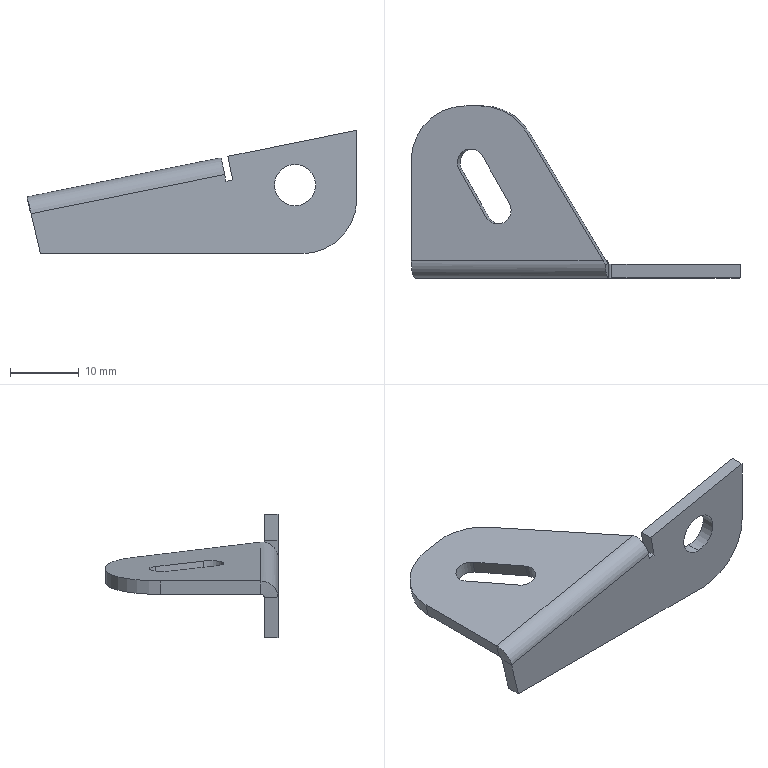Part | SolidWorks | features Fillet 3, ICE 3, Cut 1, EdgeFlange 1, FlatPattern 1, SMBaseFlange 1, SheetMetal 1 | 1 solid | 29 faces | box 48.042 x 25.072 x 17.984 mm | volume 2002 mm3 | plane 18 | cylinder 10 | spline 1 | commonest cylinder face diameters 4 x3 16 x3 6 x2 1 x1 5 x1
STEP:
#1=CARTESIAN_POINT('',(-1.659,15.796,0.3738));
#2=VERTEX_POINT('',#1);
#3=CARTESIAN_POINT('',(-5.317,14.796,-0.3654));
#4=VERTEX_POINT('',#3);
#5=CARTESIAN_POINT('',(-3.357,14.796,0.03071));
#6=DIRECTION('',(-0.1981,0.,0.9802));
#7=DIRECTION('',(-0.9802,0.,-0.1981));
#8=AXIS2_PLACEMENT_3D('',#5,#6,#7);
#9=CIRCLE('',#8,2.);
#10=EDGE_CURVE('',#2,#4,#9,.T.);
#11=ORIENTED_EDGE('',*,*,#10,.T.);
#12=CARTESIAN_POINT('',(-4.921,14.796,-2.326));
#13=VERTEX_POINT('',#12);
#14=CARTESIAN_POINT('',(-6.902,14.796,7.476));
#15=DIRECTION('',(0.1981,0.,-0.9802));
#16=VECTOR('',#15,1000.);
#17=LINE('',#14,#16);
#18=EDGE_CURVE('',#4,#13,#17,.T.);
#19=ORIENTED_EDGE('',*,*,#18,.T.);
#20=CARTESIAN_POINT('',(-1.263,15.796,-1.587));
#21=VERTEX_POINT('',#20);
#22=CARTESIAN_POINT('',(-2.961,14.796,-1.93));
#23=DIRECTION('',(-0.1981,0.,0.9802));
#24=DIRECTION('',(0.9802,0.,0.1981));
#25=AXIS2_PLACEMENT_3D('',#22,#23,#24);
#26=CIRCLE('',#25,2.);
#27=EDGE_CURVE('',#21,#13,#26,.T.);
#28=ORIENTED_EDGE('',*,*,#27,.F.);
#29=CARTESIAN_POINT('',(-3.244,15.796,8.215));
#30=DIRECTION('',(0.1981,0.,-0.9802));
#31=VECTOR('',#30,1000.);
#32=LINE('',#29,#31);
#33=EDGE_CURVE('',#2,#21,#32,.T.);
#34=ORIENTED_EDGE('',*,*,#33,.F.);
#35=EDGE_LOOP('',(#11,#19,#28,#34));
#36=FACE_OUTER_BOUND('',#35,.T.);
#37=CARTESIAN_POINT('',(-4.941,14.796,7.872));
#38=DIRECTION('',(0.1981,0.,-0.9802));
#39=DIRECTION('',(-0.9802,0.,-0.1981));
#40=AXIS2_PLACEMENT_3D('',#37,#38,#39);
#41=CYLINDRICAL_SURFACE('',#40,2.);
#42=ADVANCED_FACE('',(#36),#41,.F.);
#43=CARTESIAN_POINT('',(27.,-2.,-3.));
#44=VERTEX_POINT('',#43);
#45=CARTESIAN_POINT('',(27.,-2.,3.));
#46=VERTEX_POINT('',#45);
#47=CARTESIAN_POINT('',(27.,-2.,0.));
#48=DIRECTION('',(0.,1.,0.));
#49=DIRECTION('',(0.,0.,1.));
#50=AXIS2_PLACEMENT_3D('',#47,#48,#49);
#51=CIRCLE('',#50,3.);
#52=EDGE_CURVE('',#44,#46,#51,.T.);
#53=ORIENTED_EDGE('',*,*,#52,.F.);
#54=CARTESIAN_POINT('',(27.,0.,-3.));
#55=VERTEX_POINT('',#54);
#56=CARTESIAN_POINT('',(27.,-2.,-3.));
#57=DIRECTION('',(0.,1.,0.));
#58=VECTOR('',#57,1000.);
#59=LINE('',#56,#58);
#60=EDGE_CURVE('',#44,#55,#59,.T.);
#61=ORIENTED_EDGE('',*,*,#60,.T.);
#62=CARTESIAN_POINT('',(27.,0.,3.));
#63=VERTEX_POINT('',#62);
#64=CARTESIAN_POINT('',(27.,0.,0.));
#65=DIRECTION('',(0.,1.,0.));
#66=DIRECTION('',(0.,0.,1.));
#67=AXIS2_PLACEMENT_3D('',#64,#65,#66);
#68=CIRCLE('',#67,3.);
#69=EDGE_CURVE('',#55,#63,#68,.T.);
#70=ORIENTED_EDGE('',*,*,#69,.T.);
#71=CARTESIAN_POINT('',(27.,-2.,3.));
#72=DIRECTION('',(0.,1.,0.));
#73=VECTOR('',#72,1000.);
#74=LINE('',#71,#73);
#75=EDGE_CURVE('',#46,#63,#74,.T.);
#76=ORIENTED_EDGE('',*,*,#75,.F.);
#77=EDGE_LOOP('',(#53,#61,#70,#76));
#78=FACE_OUTER_BOUND('',#77,.T.);
#79=CARTESIAN_POINT('',(27.,-2.,0.));
#80=DIRECTION('',(0.,1.,0.));
#81=DIRECTION('',(0.,0.,1.));
#82=AXIS2_PLACEMENT_3D('',#79,#80,#81);
#83=CYLINDRICAL_SURFACE('',#82,3.);
#84=ADVANCED_FACE('',(#78),#83,.F.);
#85=CARTESIAN_POINT('',(15.931,0.5,3.928));
#86=VERTEX_POINT('',#85);
#87=CARTESIAN_POINT('',(4.775,19.227,1.674));
#88=VERTEX_POINT('',#87);
#89=CARTESIAN_POINT('',(11.814,7.411,3.096));
#90=DIRECTION('',(-0.5091,0.8545,-0.1029));
#91=VECTOR('',#90,1000.);
#92=LINE('',#89,#91);
#93=EDGE_CURVE('',#86,#88,#92,.T.);
#94=ORIENTED_EDGE('',*,*,#93,.T.);
#95=CARTESIAN_POINT('',(-1.926,23.072,0.3199));
#96=VERTEX_POINT('',#95);
#97=CARTESIAN_POINT('',(-1.926,15.072,0.3199));
#98=DIRECTION('',(-0.1981,0.,0.9802));
#99=DIRECTION('',(-0.9802,0.,-0.1981));
#100=AXIS2_PLACEMENT_3D('',#97,#98,#99);
#101=CIRCLE('',#100,8.);
#102=EDGE_CURVE('',#88,#96,#101,.T.);
#103=ORIENTED_EDGE('',*,*,#102,.T.);
#104=CARTESIAN_POINT('',(-4.201,23.072,-0.1398));
#105=VERTEX_POINT('',#104);
#106=CARTESIAN_POINT('',(-12.042,23.072,-1.724));
#107=DIRECTION('',(0.9802,0.,0.1981));
#108=VECTOR('',#107,1000.);
#109=LINE('',#106,#108);
#110=EDGE_CURVE('',#105,#96,#109,.T.);
#111=ORIENTED_EDGE('',*,*,#110,.F.);
#112=CARTESIAN_POINT('',(-12.042,15.072,-1.724));
#113=VERTEX_POINT('',#112);
#114=CARTESIAN_POINT('',(-4.201,15.072,-0.1398));
#115=DIRECTION('',(-0.1981,0.,0.9802));
#116=DIRECTION('',(-0.9802,0.,-0.1981));
#117=AXIS2_PLACEMENT_3D('',#114,#115,#116);
#118=CIRCLE('',#117,8.);
#119=EDGE_CURVE('',#105,#113,#118,.T.);
#120=ORIENTED_EDGE('',*,*,#119,.T.);
#121=CARTESIAN_POINT('',(-12.042,0.5,-1.724));
#122=VERTEX_POINT('',#121);
#123=CARTESIAN_POINT('',(-12.042,0.,-1.724));
#124=DIRECTION('',(0.,1.,0.));
#125=VECTOR('',#124,1000.);
#126=LINE('',#123,#125);
#127=EDGE_CURVE('',#122,#113,#126,.T.);
#128=ORIENTED_EDGE('',*,*,#127,.F.);
#129=CARTESIAN_POINT('',(-12.042,0.5,-1.724));
#130=DIRECTION('',(-0.9802,0.,-0.1981));
#131=VECTOR('',#130,1000.);
#132=LINE('',#129,#131);
#133=EDGE_CURVE('',#86,#122,#132,.T.);
#134=ORIENTED_EDGE('',*,*,#133,.F.);
#135=EDGE_LOOP('',(#94,#103,#111,#120,#128,#134));
#136=FACE_OUTER_BOUND('',#135,.T.);
#137=ORIENTED_EDGE('',*,*,#10,.F.);
#138=CARTESIAN_POINT('',(2.262,8.867,1.166));
#139=VERTEX_POINT('',#138);
#140=CARTESIAN_POINT('',(5.425,3.277,1.805));
#141=DIRECTION('',(-0.4901,0.866,-0.09904));
#142=VECTOR('',#141,1000.);
#143=LINE('',#140,#142);
#144=EDGE_CURVE('',#139,#2,#143,.T.);
#145=ORIENTED_EDGE('',*,*,#144,.F.);
#146=CARTESIAN_POINT('',(-1.134,6.867,0.4799));
#147=VERTEX_POINT('',#146);
#148=CARTESIAN_POINT('',(0.564,7.867,0.823));
#149=DIRECTION('',(-0.1981,0.,0.9802));
#150=DIRECTION('',(-0.9802,0.,-0.1981));
#151=AXIS2_PLACEMENT_3D('',#148,#149,#150);
#152=CIRCLE('',#151,2.);
#153=EDGE_CURVE('',#147,#139,#152,.T.);
#154=ORIENTED_EDGE('',*,*,#153,.F.);
#155=CARTESIAN_POINT('',(-5.055,13.796,-0.3124));
#156=VERTEX_POINT('',#155);
#157=CARTESIAN_POINT('',(2.03,1.277,1.119));
#158=DIRECTION('',(0.4901,-0.866,0.09904));
#159=VECTOR('',#158,1000.);
#160=LINE('',#157,#159);
#161=EDGE_CURVE('',#156,#147,#160,.T.);
#162=ORIENTED_EDGE('',*,*,#161,.F.);
#163=CARTESIAN_POINT('',(-3.357,14.796,0.03071));
#164=DIRECTION('',(-0.1981,0.,0.9802));
#165=DIRECTION('',(-0.9802,0.,-0.1981));
#166=AXIS2_PLACEMENT_3D('',#163,#164,#165);
#167=CIRCLE('',#166,2.);
#168=EDGE_CURVE('',#4,#156,#167,.T.);
#169=ORIENTED_EDGE('',*,*,#168,.F.);
#170=EDGE_LOOP('',(#137,#145,#154,#162,#169));
#171=FACE_BOUND('',#170,.T.);
#172=CARTESIAN_POINT('',(-0.1377,0.,0.6812));
#173=DIRECTION('',(0.1981,0.,-0.9802));
#174=DIRECTION('',(-0.9802,0.,-0.1981));
#175=AXIS2_PLACEMENT_3D('',#172,#173,#174);
#176=PLANE('',#175);
#177=ADVANCED_FACE('',(#136,#171),#176,.F.);
#178=CARTESIAN_POINT('',(-3.805,23.072,-2.1));
#179=VERTEX_POINT('',#178);
#180=CARTESIAN_POINT('',(-1.53,23.072,-1.64));
#181=VERTEX_POINT('',#180);
#182=CARTESIAN_POINT('',(0.2585,23.072,-1.279));
#183=DIRECTION('',(0.9802,0.,0.1981));
#184=VECTOR('',#183,1000.);
#185=LINE('',#182,#184);
#186=EDGE_CURVE('',#179,#181,#185,.T.);
#187=ORIENTED_EDGE('',*,*,#186,.T.);
#188=CARTESIAN_POINT('',(5.171,19.227,-0.2864));
#189=VERTEX_POINT('',#188);
#190=CARTESIAN_POINT('',(-1.53,15.072,-1.64));
#191=DIRECTION('',(0.1981,0.,-0.9802));
#192=DIRECTION('',(-0.9802,0.,-0.1981));
#193=AXIS2_PLACEMENT_3D('',#190,#191,#192);
#194=CIRCLE('',#193,8.);
#195=EDGE_CURVE('',#181,#189,#194,.T.);
#196=ORIENTED_EDGE('',*,*,#195,.T.);
#197=CARTESIAN_POINT('',(16.327,0.5,1.968));
#198=VERTEX_POINT('',#197);
#199=CARTESIAN_POINT('',(16.625,0.,2.028));
#200=DIRECTION('',(-0.5091,0.8545,-0.1029));
#201=VECTOR('',#200,1000.);
#202=LINE('',#199,#201);
#203=EDGE_CURVE('',#198,#189,#202,.T.);
#204=ORIENTED_EDGE('',*,*,#203,.F.);
#205=CARTESIAN_POINT('',(-11.646,0.5,-3.685));
#206=VERTEX_POINT('',#205);
#207=CARTESIAN_POINT('',(-11.646,0.5,-3.685));
#208=DIRECTION('',(0.9802,0.,0.1981));
#209=VECTOR('',#208,1000.);
#210=LINE('',#207,#209);
#211=EDGE_CURVE('',#206,#198,#210,.T.);
#212=ORIENTED_EDGE('',*,*,#211,.F.);
#213=CARTESIAN_POINT('',(-11.646,15.072,-3.685));
#214=VERTEX_POINT('',#213);
#215=CARTESIAN_POINT('',(-11.646,0.,-3.685));
#216=DIRECTION('',(0.,1.,0.));
#217=VECTOR('',#216,1000.);
#218=LINE('',#215,#217);
#219=EDGE_CURVE('',#206,#214,#218,.T.);
#220=ORIENTED_EDGE('',*,*,#219,.T.);
#221=CARTESIAN_POINT('',(-3.805,15.072,-2.1));
#222=DIRECTION('',(0.1981,0.,-0.9802));
#223=DIRECTION('',(-0.9802,0.,-0.1981));
#224=AXIS2_PLACEMENT_3D('',#221,#222,#223);
#225=CIRCLE('',#224,8.);
#226=EDGE_CURVE('',#214,#179,#225,.T.);
#227=ORIENTED_EDGE('',*,*,#226,.T.);
#228=EDGE_LOOP('',(#187,#196,#204,#212,#220,#227));
#229=FACE_OUTER_BOUND('',#228,.T.);
#230=CARTESIAN_POINT('',(2.658,8.867,-0.7943));
#231=VERTEX_POINT('',#230);
#232=CARTESIAN_POINT('',(-1.263,15.796,-1.587));
#233=DIRECTION('',(-0.4901,0.866,-0.09904));
#234=VECTOR('',#233,1000.);
#235=LINE('',#232,#234);
#236=EDGE_CURVE('',#231,#21,#235,.T.);
#237=ORIENTED_EDGE('',*,*,#236,.T.);
#238=ORIENTED_EDGE('',*,*,#27,.T.);
#239=CARTESIAN_POINT('',(-4.658,13.796,-2.273));
#240=VERTEX_POINT('',#239);
#241=CARTESIAN_POINT('',(-2.961,14.796,-1.93));
#242=DIRECTION('',(-0.1981,0.,0.9802));
#243=DIRECTION('',(0.9802,0.,0.1981));
#244=AXIS2_PLACEMENT_3D('',#241,#242,#243);
#245=CIRCLE('',#244,2.);
#246=EDGE_CURVE('',#13,#240,#245,.T.);
#247=ORIENTED_EDGE('',*,*,#246,.T.);
#248=CARTESIAN_POINT('',(-0.7376,6.867,-1.48));
#249=VERTEX_POINT('',#248);
#250=CARTESIAN_POINT('',(-4.658,13.796,-2.273));
#251=DIRECTION('',(0.4901,-0.866,0.09904));
#252=VECTOR('',#251,1000.);
#253=LINE('',#250,#252);
#254=EDGE_CURVE('',#240,#249,#253,.T.);
#255=ORIENTED_EDGE('',*,*,#254,.T.);
#256=CARTESIAN_POINT('',(0.9601,7.867,-1.137));
#257=DIRECTION('',(-0.1981,0.,0.9802));
#258=DIRECTION('',(0.9802,0.,0.1981));
#259=AXIS2_PLACEMENT_3D('',#256,#257,#258);
#260=CIRCLE('',#259,2.);
#261=EDGE_CURVE('',#249,#231,#260,.T.);
#262=ORIENTED_EDGE('',*,*,#261,.T.);
#263=EDGE_LOOP('',(#237,#238,#247,#255,#262));
#264=FACE_BOUND('',#263,.T.);
#265=CARTESIAN_POINT('',(0.2585,0.,-1.279));
#266=DIRECTION('',(0.1981,0.,-0.9802));
#267=DIRECTION('',(-0.9802,0.,-0.1981));
#268=AXIS2_PLACEMENT_3D('',#265,#266,#267);
#269=PLANE('',#268);
#270=ADVANCED_FACE('',(#229,#264),#269,.T.);
#271=CARTESIAN_POINT('',(27.,-2.,0.));
#272=DIRECTION('',(0.,1.,0.));
#273=DIRECTION('',(0.,0.,1.));
#274=AXIS2_PLACEMENT_3D('',#271,#272,#273);
#275=CIRCLE('',#274,3.);
#276=EDGE_CURVE('',#46,#44,#275,.T.);
#277=ORIENTED_EDGE('',*,*,#276,.T.);
#278=ORIENTED_EDGE('',*,*,#52,.T.);
#279=EDGE_LOOP('',(#277,#278));
#280=FACE_BOUND('',#279,.T.);
#281=CARTESIAN_POINT('',(28.,-2.,-10.));
#282=VERTEX_POINT('',#281);
#283=CARTESIAN_POINT('',(-10.106,-2.,-10.));
#284=VERTEX_POINT('',#283);
#285=CARTESIAN_POINT('',(-36.,-2.,-10.));
#286=DIRECTION('',(-1.,0.,0.));
#287=VECTOR('',#286,1000.);
#288=LINE('',#285,#287);
#289=EDGE_CURVE('',#282,#284,#288,.T.);
#290=ORIENTED_EDGE('',*,*,#289,.F.);
#291=CARTESIAN_POINT('',(36.,-2.,-2.));
#292=VERTEX_POINT('',#291);
#293=CARTESIAN_POINT('',(28.,-2.,-2.));
#294=DIRECTION('',(0.,-1.,0.));
#295=DIRECTION('',(0.,0.,1.));
#296=AXIS2_PLACEMENT_3D('',#293,#294,#295);
#297=CIRCLE('',#296,8.);
#298=EDGE_CURVE('',#282,#292,#297,.T.);
#299=ORIENTED_EDGE('',*,*,#298,.T.);
#300=CARTESIAN_POINT('',(36.,-2.,7.984));
#301=VERTEX_POINT('',#300);
#302=CARTESIAN_POINT('',(36.,-2.,-10.));
#303=DIRECTION('',(0.,0.,-1.));
#304=VECTOR('',#303,1000.);
#305=LINE('',#302,#304);
#306=EDGE_CURVE('',#301,#292,#305,.T.);
#307=ORIENTED_EDGE('',*,*,#306,.F.);
#308=CARTESIAN_POINT('',(17.209,-2.,4.187));
#309=VERTEX_POINT('',#308);
#310=CARTESIAN_POINT('',(-0.1377,-2.,0.6812));
#311=DIRECTION('',(0.9802,0.,0.1981));
#312=VECTOR('',#311,1000.);
#313=LINE('',#310,#312);
#314=EDGE_CURVE('',#309,#301,#313,.T.);
#315=ORIENTED_EDGE('',*,*,#314,.F.);
#316=CARTESIAN_POINT('',(17.903,-2.,0.756));
#317=VERTEX_POINT('',#316);
#318=CARTESIAN_POINT('',(17.347,-2.,3.505));
#319=DIRECTION('',(-0.1981,0.,0.9802));
#320=VECTOR('',#319,1000.);
#321=LINE('',#318,#320);
#322=EDGE_CURVE('',#317,#309,#321,.T.);
#323=ORIENTED_EDGE('',*,*,#322,.F.);
#324=CARTESIAN_POINT('',(16.922,-2.,0.558));
#325=VERTEX_POINT('',#324);
#326=CARTESIAN_POINT('',(0.5556,-2.,-2.749));
#327=DIRECTION('',(0.9802,0.,0.1981));
#328=VECTOR('',#327,1000.);
#329=LINE('',#326,#328);
#330=EDGE_CURVE('',#325,#317,#329,.T.);
#331=ORIENTED_EDGE('',*,*,#330,.F.);
#332=CARTESIAN_POINT('',(16.724,-2.,1.538));
#333=VERTEX_POINT('',#332);
#334=CARTESIAN_POINT('',(16.367,-2.,3.307));
#335=DIRECTION('',(0.1981,0.,-0.9802));
#336=VECTOR('',#335,1000.);
#337=LINE('',#334,#336);
#338=EDGE_CURVE('',#333,#325,#337,.T.);
#339=ORIENTED_EDGE('',*,*,#338,.F.);
#340=CARTESIAN_POINT('',(-11.473,-2.,-4.16));
#341=VERTEX_POINT('',#340);
#342=CARTESIAN_POINT('',(16.724,-2.,1.538));
#343=DIRECTION('',(-0.9802,0.,-0.1981));
#344=VECTOR('',#343,1000.);
#345=LINE('',#342,#344);
#346=EDGE_CURVE('',#333,#341,#345,.T.);
#347=ORIENTED_EDGE('',*,*,#346,.T.);
#348=CARTESIAN_POINT('',(-11.8,-2.,-2.76));
#349=DIRECTION('',(0.2278,0.,-0.9737));
#350=VECTOR('',#349,1000.);
#351=LINE('',#348,#350);
#352=EDGE_CURVE('',#341,#284,#351,.T.);
#353=ORIENTED_EDGE('',*,*,#352,.T.);
#354=EDGE_LOOP('',(#290,#299,#307,#315,#323,#331,#339,#347,#353));
#355=FACE_OUTER_BOUND('',#354,.T.);
#356=CARTESIAN_POINT('',(0.,-2.,0.));
#357=DIRECTION('',(0.,1.,0.));
#358=DIRECTION('',(0.,0.,1.));
#359=AXIS2_PLACEMENT_3D('',#356,#357,#358);
#360=PLANE('',#359);
#361=ADVANCED_FACE('',(#280,#355),#360,.F.);
#362=CARTESIAN_POINT('',(27.,0.,0.));
#363=DIRECTION('',(0.,1.,0.));
#364=DIRECTION('',(0.,0.,1.));
#365=AXIS2_PLACEMENT_3D('',#362,#363,#364);
#366=CIRCLE('',#365,3.);
#367=EDGE_CURVE('',#63,#55,#366,.T.);
#368=ORIENTED_EDGE('',*,*,#367,.F.);
#369=ORIENTED_EDGE('',*,*,#69,.F.);
#370=EDGE_LOOP('',(#368,#369));
#371=FACE_BOUND('',#370,.T.);
#372=CARTESIAN_POINT('',(36.,0.,7.984));
#373=VERTEX_POINT('',#372);
#374=CARTESIAN_POINT('',(36.,0.,-2.));
#375=VERTEX_POINT('',#374);
#376=CARTESIAN_POINT('',(36.,0.,-10.));
#377=DIRECTION('',(0.,0.,-1.));
#378=VECTOR('',#377,1000.);
#379=LINE('',#376,#378);
#380=EDGE_CURVE('',#373,#375,#379,.T.);
#381=ORIENTED_EDGE('',*,*,#380,.T.);
#382=CARTESIAN_POINT('',(28.,0.,-10.));
#383=VERTEX_POINT('',#382);
#384=CARTESIAN_POINT('',(28.,0.,-2.));
#385=DIRECTION('',(0.,1.,0.));
#386=DIRECTION('',(0.,0.,1.));
#387=AXIS2_PLACEMENT_3D('',#384,#385,#386);
#388=CIRCLE('',#387,8.);
#389=EDGE_CURVE('',#375,#383,#388,.T.);
#390=ORIENTED_EDGE('',*,*,#389,.T.);
#391=CARTESIAN_POINT('',(-10.106,0.,-10.));
#392=VERTEX_POINT('',#391);
#393=CARTESIAN_POINT('',(-36.,0.,-10.));
#394=DIRECTION('',(-1.,0.,0.));
#395=VECTOR('',#394,1000.);
#396=LINE('',#393,#395);
#397=EDGE_CURVE('',#383,#392,#396,.T.);
#398=ORIENTED_EDGE('',*,*,#397,.T.);
#399=CARTESIAN_POINT('',(-11.473,0.,-4.16));
#400=VERTEX_POINT('',#399);
#401=CARTESIAN_POINT('',(-11.8,0.,-2.76));
#402=DIRECTION('',(0.2278,0.,-0.9737));
#403=VECTOR('',#402,1000.);
#404=LINE('',#401,#403);
#405=EDGE_CURVE('',#400,#392,#404,.T.);
#406=ORIENTED_EDGE('',*,*,#405,.F.);
#407=CARTESIAN_POINT('',(16.724,0.,1.538));
#408=VERTEX_POINT('',#407);
#409=CARTESIAN_POINT('',(16.724,0.,1.538));
#410=DIRECTION('',(-0.9802,0.,-0.1981));
#411=VECTOR('',#410,1000.);
#412=LINE('',#409,#411);
#413=EDGE_CURVE('',#408,#400,#412,.T.);
#414=ORIENTED_EDGE('',*,*,#413,.F.);
#415=CARTESIAN_POINT('',(16.922,0.,0.558));
#416=VERTEX_POINT('',#415);
#417=CARTESIAN_POINT('',(16.922,0.,0.558));
#418=DIRECTION('',(-0.1981,0.,0.9802));
#419=VECTOR('',#418,1000.);
#420=LINE('',#417,#419);
#421=EDGE_CURVE('',#416,#408,#420,.T.);
#422=ORIENTED_EDGE('',*,*,#421,.F.);
#423=CARTESIAN_POINT('',(17.903,0.,0.756));
#424=VERTEX_POINT('',#423);
#425=CARTESIAN_POINT('',(17.903,0.,0.756));
#426=DIRECTION('',(-0.9802,0.,-0.1981));
#427=VECTOR('',#426,1000.);
#428=LINE('',#425,#427);
#429=EDGE_CURVE('',#424,#416,#428,.T.);
#430=ORIENTED_EDGE('',*,*,#429,.F.);
#431=CARTESIAN_POINT('',(17.209,0.,4.187));
#432=VERTEX_POINT('',#431);
#433=CARTESIAN_POINT('',(17.209,0.,4.187));
#434=DIRECTION('',(0.1981,0.,-0.9802));
#435=VECTOR('',#434,1000.);
#436=LINE('',#433,#435);
#437=EDGE_CURVE('',#432,#424,#436,.T.);
#438=ORIENTED_EDGE('',*,*,#437,.F.);
#439=CARTESIAN_POINT('',(-0.1377,0.,0.6812));
#440=DIRECTION('',(0.9802,0.,0.1981));
#441=VECTOR('',#440,1000.);
#442=LINE('',#439,#441);
#443=EDGE_CURVE('',#432,#373,#442,.T.);
#444=ORIENTED_EDGE('',*,*,#443,.T.);
#445=EDGE_LOOP('',(#381,#390,#398,#406,#414,#422,#430,#438,#444));
#446=FACE_OUTER_BOUND('',#445,.T.);
#447=CARTESIAN_POINT('',(0.,0.,0.));
#448=DIRECTION('',(0.,1.,0.));
#449=DIRECTION('',(0.,0.,1.));
#450=AXIS2_PLACEMENT_3D('',#447,#448,#449);
#451=PLANE('',#450);
#452=ADVANCED_FACE('',(#371,#446),#451,.T.);
#453=ORIENTED_EDGE('',*,*,#443,.F.);
#454=CARTESIAN_POINT('',(17.209,0.,4.187));
#455=DIRECTION('',(0.,-1.,0.));
#456=VECTOR('',#455,1000.);
#457=LINE('',#454,#456);
#458=EDGE_CURVE('',#432,#309,#457,.T.);
#459=ORIENTED_EDGE('',*,*,#458,.T.);
#460=ORIENTED_EDGE('',*,*,#314,.T.);
#461=CARTESIAN_POINT('',(36.,-10.,7.984));
#462=DIRECTION('',(0.,1.,0.));
#463=VECTOR('',#462,1000.);
#464=LINE('',#461,#463);
#465=EDGE_CURVE('',#301,#373,#464,.T.);
#466=ORIENTED_EDGE('',*,*,#465,.T.);
#467=EDGE_LOOP('',(#453,#459,#460,#466));
#468=FACE_OUTER_BOUND('',#467,.T.);
#469=CARTESIAN_POINT('',(-0.1377,-10.,0.6812));
#470=DIRECTION('',(-0.1981,0.,0.9802));
#471=DIRECTION('',(0.9802,0.,0.1981));
#472=AXIS2_PLACEMENT_3D('',#469,#470,#471);
#473=PLANE('',#472);
#474=ADVANCED_FACE('',(#468),#473,.T.);
#475=CARTESIAN_POINT('',(-11.473,0.,-4.16));
#476=DIRECTION('',(0.,-1.,0.));
#477=VECTOR('',#476,1000.);
#478=LINE('',#475,#477);
#479=EDGE_CURVE('',#400,#341,#478,.T.);
#480=ORIENTED_EDGE('',*,*,#479,.F.);
#481=ORIENTED_EDGE('',*,*,#405,.T.);
#482=CARTESIAN_POINT('',(-10.106,-10.,-10.));
#483=DIRECTION('',(0.,1.,0.));
#484=VECTOR('',#483,1000.);
#485=LINE('',#482,#484);
#486=EDGE_CURVE('',#284,#392,#485,.T.);
#487=ORIENTED_EDGE('',*,*,#486,.F.);
#488=ORIENTED_EDGE('',*,*,#352,.F.);
#489=EDGE_LOOP('',(#480,#481,#487,#488));
#490=FACE_OUTER_BOUND('',#489,.T.);
#491=CARTESIAN_POINT('',(-11.8,-10.,-2.76));
#492=DIRECTION('',(0.9737,0.,0.2278));
#493=DIRECTION('',(0.2278,0.,-0.9737));
#494=AXIS2_PLACEMENT_3D('',#491,#492,#493);
#495=PLANE('',#494);
#496=ADVANCED_FACE('',(#490),#495,.F.);
#497=ORIENTED_EDGE('',*,*,#306,.T.);
#498=CARTESIAN_POINT('',(36.,-2.,-2.));
#499=DIRECTION('',(0.,1.,0.));
#500=VECTOR('',#499,1000.);
#501=LINE('',#498,#500);
#502=EDGE_CURVE('',#292,#375,#501,.T.);
#503=ORIENTED_EDGE('',*,*,#502,.T.);
#504=ORIENTED_EDGE('',*,*,#380,.F.);
#505=ORIENTED_EDGE('',*,*,#465,.F.);
#506=EDGE_LOOP('',(#497,#503,#504,#505));
#507=FACE_OUTER_BOUND('',#506,.T.);
#508=CARTESIAN_POINT('',(36.,-2.,-10.));
#509=DIRECTION('',(1.,0.,0.));
#510=DIRECTION('',(0.,0.,-1.));
#511=AXIS2_PLACEMENT_3D('',#508,#509,#510);
#512=PLANE('',#511);
#513=ADVANCED_FACE('',(#507),#512,.T.);
#514=ORIENTED_EDGE('',*,*,#397,.F.);
#515=CARTESIAN_POINT('',(28.,-2.,-10.));
#516=DIRECTION('',(0.,-1.,0.));
#517=VECTOR('',#516,1000.);
#518=LINE('',#515,#517);
#519=EDGE_CURVE('',#383,#282,#518,.T.);
#520=ORIENTED_EDGE('',*,*,#519,.T.);
#521=ORIENTED_EDGE('',*,*,#289,.T.);
#522=ORIENTED_EDGE('',*,*,#486,.T.);
#523=EDGE_LOOP('',(#514,#520,#521,#522));
#524=FACE_OUTER_BOUND('',#523,.T.);
#525=CARTESIAN_POINT('',(-36.,-2.,-10.));
#526=DIRECTION('',(0.,0.,-1.));
#527=DIRECTION('',(-1.,0.,0.));
#528=AXIS2_PLACEMENT_3D('',#525,#526,#527);
#529=PLANE('',#528);
#530=ADVANCED_FACE('',(#524),#529,.T.);
#531=ORIENTED_EDGE('',*,*,#60,.F.);
#532=ORIENTED_EDGE('',*,*,#276,.F.);
#533=ORIENTED_EDGE('',*,*,#75,.T.);
#534=ORIENTED_EDGE('',*,*,#367,.T.);
#535=EDGE_LOOP('',(#531,#532,#533,#534));
#536=FACE_OUTER_BOUND('',#535,.T.);
#537=CARTESIAN_POINT('',(27.,-2.,0.));
#538=DIRECTION('',(0.,1.,0.));
#539=DIRECTION('',(0.,0.,1.));
#540=AXIS2_PLACEMENT_3D('',#537,#538,#539);
#541=CYLINDRICAL_SURFACE('',#540,3.);
#542=ADVANCED_FACE('',(#536),#541,.F.);
#543=CARTESIAN_POINT('',(16.922,0.,0.558));
#544=DIRECTION('',(0.,-1.,0.));
#545=VECTOR('',#544,1000.);
#546=LINE('',#543,#545);
#547=EDGE_CURVE('',#416,#325,#546,.T.);
#548=ORIENTED_EDGE('',*,*,#547,.T.);
#549=ORIENTED_EDGE('',*,*,#330,.T.);
#550=CARTESIAN_POINT('',(17.903,0.,0.756));
#551=DIRECTION('',(0.,-1.,0.));
#552=VECTOR('',#551,1000.);
#553=LINE('',#550,#552);
#554=EDGE_CURVE('',#424,#317,#553,.T.);
#555=ORIENTED_EDGE('',*,*,#554,.F.);
#556=ORIENTED_EDGE('',*,*,#429,.T.);
#557=EDGE_LOOP('',(#548,#549,#555,#556));
#558=FACE_OUTER_BOUND('',#557,.T.);
#559=CARTESIAN_POINT('',(17.903,0.,0.756));
#560=DIRECTION('',(-0.1981,0.,0.9802));
#561=DIRECTION('',(0.9802,0.,0.1981));
#562=AXIS2_PLACEMENT_3D('',#559,#560,#561);
#563=PLANE('',#562);
#564=ADVANCED_FACE('',(#558),#563,.T.);
#565=CARTESIAN_POINT('',(16.724,0.,1.538));
#566=DIRECTION('',(0.,-1.,0.));
#567=VECTOR('',#566,1000.);
#568=LINE('',#565,#567);
#569=EDGE_CURVE('',#408,#333,#568,.T.);
#570=ORIENTED_EDGE('',*,*,#569,.T.);
#571=ORIENTED_EDGE('',*,*,#338,.T.);
#572=ORIENTED_EDGE('',*,*,#547,.F.);
#573=ORIENTED_EDGE('',*,*,#421,.T.);
#574=EDGE_LOOP('',(#570,#571,#572,#573));
#575=FACE_OUTER_BOUND('',#574,.T.);
#576=CARTESIAN_POINT('',(16.922,0.,0.558));
#577=DIRECTION('',(0.9802,0.,0.1981));
#578=DIRECTION('',(0.1981,0.,-0.9802));
#579=AXIS2_PLACEMENT_3D('',#576,#577,#578);
#580=PLANE('',#579);
#581=ADVANCED_FACE('',(#575),#580,.T.);
#582=ORIENTED_EDGE('',*,*,#554,.T.);
#583=ORIENTED_EDGE('',*,*,#322,.T.);
#584=ORIENTED_EDGE('',*,*,#458,.F.);
#585=ORIENTED_EDGE('',*,*,#437,.T.);
#586=EDGE_LOOP('',(#582,#583,#584,#585));
#587=FACE_OUTER_BOUND('',#586,.T.);
#588=CARTESIAN_POINT('',(17.209,0.,4.187));
#589=DIRECTION('',(-0.9802,0.,-0.1981));
#590=DIRECTION('',(-0.1981,0.,0.9802));
#591=AXIS2_PLACEMENT_3D('',#588,#589,#590);
#592=PLANE('',#591);
#593=ADVANCED_FACE('',(#587),#592,.T.);
#594=CARTESIAN_POINT('',(-12.042,0.5,-1.724));
#595=DIRECTION('',(-0.1981,0.,0.9802));
#596=VECTOR('',#595,1000.);
#597=LINE('',#594,#596);
#598=EDGE_CURVE('',#206,#122,#597,.T.);
#599=ORIENTED_EDGE('',*,*,#598,.F.);
#600=CARTESIAN_POINT('',(-11.473,0.,-4.16));
#601=CARTESIAN_POINT('',(-11.511,0.,-4.034));
#602=CARTESIAN_POINT('',(-11.549,0.05389,-3.909));
#603=CARTESIAN_POINT('',(-11.611,0.239,-3.733));
#604=CARTESIAN_POINT('',(-11.634,0.3691,-3.682));
#605=CARTESIAN_POINT('',(-11.646,0.5,-3.685));
#606=B_SPLINE_CURVE_WITH_KNOTS('',3,(#600,#601,#602,#603,#604,#605),.UNSPECIFIED.,.F.,.F.,(4,2,4),(0.,0.5,1.),.UNSPECIFIED.);
#607=EDGE_CURVE('',#400,#206,#606,.T.);
#608=ORIENTED_EDGE('',*,*,#607,.F.);
#609=ORIENTED_EDGE('',*,*,#479,.T.);
#610=CARTESIAN_POINT('',(-11.473,-2.,-4.16));
#611=CARTESIAN_POINT('',(-11.544,-2.,-3.84));
#612=CARTESIAN_POINT('',(-11.615,-1.935,-3.521));
#613=CARTESIAN_POINT('',(-11.747,-1.684,-2.931));
#614=CARTESIAN_POINT('',(-11.808,-1.499,-2.66));
#615=CARTESIAN_POINT('',(-11.912,-1.036,-2.209));
#616=CARTESIAN_POINT('',(-11.955,-0.759,-2.029));
#617=CARTESIAN_POINT('',(-12.017,-0.1544,-1.786));
#618=CARTESIAN_POINT('',(-12.036,0.1728,-1.723));
#619=CARTESIAN_POINT('',(-12.042,0.5,-1.724));
#620=B_SPLINE_CURVE_WITH_KNOTS('',3,(#610,#611,#612,#613,#614,#615,#616,#617,#618,#619),.UNSPECIFIED.,.F.,.F.,(4,2,2,2,4),(0.,0.25,0.5,0.75,1.),.UNSPECIFIED.);
#621=EDGE_CURVE('',#341,#122,#620,.T.);
#622=ORIENTED_EDGE('',*,*,#621,.T.);
#623=EDGE_LOOP('',(#599,#608,#609,#622));
#624=FACE_OUTER_BOUND('',#623,.T.);
#625=CARTESIAN_POINT('',(-11.473,-2.02,-4.16));
#626=CARTESIAN_POINT('',(-11.544,-2.02,-3.838));
#627=CARTESIAN_POINT('',(-11.616,-1.954,-3.516));
#628=CARTESIAN_POINT('',(-11.749,-1.702,-2.921));
#629=CARTESIAN_POINT('',(-11.81,-1.515,-2.648));
#630=CARTESIAN_POINT('',(-11.915,-1.049,-2.193));
#631=CARTESIAN_POINT('',(-11.958,-0.7691,-2.012));
#632=CARTESIAN_POINT('',(-12.021,-0.1596,-1.767));
#633=CARTESIAN_POINT('',(-12.04,0.1701,-1.704));
#634=CARTESIAN_POINT('',(-12.046,0.5,-1.705));
#635=CARTESIAN_POINT('',(-11.473,-2.,-4.16));
#636=CARTESIAN_POINT('',(-11.544,-2.,-3.84));
#637=CARTESIAN_POINT('',(-11.615,-1.935,-3.521));
#638=CARTESIAN_POINT('',(-11.747,-1.684,-2.931));
#639=CARTESIAN_POINT('',(-11.808,-1.499,-2.66));
#640=CARTESIAN_POINT('',(-11.912,-1.036,-2.209));
#641=CARTESIAN_POINT('',(-11.955,-0.759,-2.029));
#642=CARTESIAN_POINT('',(-12.017,-0.1544,-1.786));
#643=CARTESIAN_POINT('',(-12.036,0.1727,-1.723));
#644=CARTESIAN_POINT('',(-12.042,0.5,-1.724));
#645=CARTESIAN_POINT('',(-11.473,0.,-4.16));
#646=CARTESIAN_POINT('',(-11.492,0.,-4.097));
#647=CARTESIAN_POINT('',(-11.511,0.01301,-4.034));
#648=CARTESIAN_POINT('',(-11.547,0.06311,-3.918));
#649=CARTESIAN_POINT('',(-11.564,0.1002,-3.865));
#650=CARTESIAN_POINT('',(-11.595,0.1927,-3.777));
#651=CARTESIAN_POINT('',(-11.609,0.2482,-3.742));
#652=CARTESIAN_POINT('',(-11.631,0.3691,-3.695));
#653=CARTESIAN_POINT('',(-11.64,0.4345,-3.684));
#654=CARTESIAN_POINT('',(-11.646,0.5,-3.685));
#655=CARTESIAN_POINT('',(-11.473,0.0202,-4.16));
#656=CARTESIAN_POINT('',(-11.491,0.0202,-4.1));
#657=CARTESIAN_POINT('',(-11.51,0.03269,-4.039));
#658=CARTESIAN_POINT('',(-11.545,0.08076,-3.928));
#659=CARTESIAN_POINT('',(-11.562,0.1163,-3.877));
#660=CARTESIAN_POINT('',(-11.592,0.2051,-3.793));
#661=CARTESIAN_POINT('',(-11.605,0.2584,-3.759));
#662=CARTESIAN_POINT('',(-11.627,0.3744,-3.714));
#663=CARTESIAN_POINT('',(-11.636,0.4372,-3.703));
#664=CARTESIAN_POINT('',(-11.642,0.5,-3.705));
#665=B_SPLINE_SURFACE_WITH_KNOTS('',1,3,((#625,#626,#627,#628,#629,#630,#631,#632,#633,#634),(#635,#636,#637,#638,#639,#640,#641,#642,#643,#644),(#645,#646,#647,#648,#649,#650,#651,#652,#653,#654),(#655,#656,#657,#658,#659,#660,#661,#662,#663,#664)),.UNSPECIFIED.,.F.,.F.,.F.,(2,1,1,2),(4,2,2,2,4),(-0.01,0.,1.,1.01),(0.,0.25,0.5,0.75,1.),.UNSPECIFIED.);
#666=ADVANCED_FACE('',(#624),#665,.F.);
#667=CARTESIAN_POINT('',(16.239,0.,3.939));
#668=VERTEX_POINT('',#667);
#669=CARTESIAN_POINT('',(16.625,0.,2.028));
#670=VERTEX_POINT('',#669);
#671=CARTESIAN_POINT('',(14.344,0.,13.316));
#672=DIRECTION('',(0.1981,0.,-0.9802));
#673=VECTOR('',#672,1000.);
#674=LINE('',#671,#673);
#675=EDGE_CURVE('',#668,#670,#674,.T.);
#676=ORIENTED_EDGE('',*,*,#675,.F.);
#677=CARTESIAN_POINT('',(16.724,0.5,1.538));
#678=DIRECTION('',(0.9802,0.,0.1981));
#679=DIRECTION('',(0.1981,0.,-0.9802));
#680=AXIS2_PLACEMENT_3D('',#677,#678,#679);
#681=CIRCLE('',#680,2.5);
#682=EDGE_CURVE('',#668,#333,#681,.T.);
#683=ORIENTED_EDGE('',*,*,#682,.T.);
#684=ORIENTED_EDGE('',*,*,#569,.F.);
#685=CARTESIAN_POINT('',(16.625,0.5,2.028));
#686=VERTEX_POINT('',#685);
#687=CARTESIAN_POINT('',(16.724,0.5,1.538));
#688=DIRECTION('',(0.9802,0.,0.1981));
#689=DIRECTION('',(0.1981,0.,-0.9802));
#690=AXIS2_PLACEMENT_3D('',#687,#688,#689);
#691=CIRCLE('',#690,0.5);
#692=EDGE_CURVE('',#686,#408,#691,.T.);
#693=ORIENTED_EDGE('',*,*,#692,.F.);
#694=CARTESIAN_POINT('',(16.625,23.072,2.028));
#695=DIRECTION('',(0.,-1.,0.));
#696=VECTOR('',#695,1000.);
#697=LINE('',#694,#696);
#698=EDGE_CURVE('',#686,#670,#697,.T.);
#699=ORIENTED_EDGE('',*,*,#698,.T.);
#700=EDGE_LOOP('',(#676,#683,#684,#693,#699));
#701=FACE_OUTER_BOUND('',#700,.T.);
#702=CARTESIAN_POINT('',(16.724,0.5,1.538));
#703=DIRECTION('',(-0.9802,0.,-0.1981));
#704=DIRECTION('',(-0.1981,0.,0.9802));
#705=AXIS2_PLACEMENT_3D('',#702,#703,#704);
#706=PLANE('',#705);
#707=ADVANCED_FACE('',(#701),#706,.F.);
#708=CARTESIAN_POINT('',(15.931,0.5,3.928));
#709=CARTESIAN_POINT('',(16.031,0.3319,3.949));
#710=CARTESIAN_POINT('',(16.134,0.1647,3.952));
#711=CARTESIAN_POINT('',(16.239,0.,3.939));
#712=(BOUNDED_CURVE()B_SPLINE_CURVE(3,(#708,#709,#710,#711),.UNSPECIFIED.,.F.,.F.)B_SPLINE_CURVE_WITH_KNOTS((4,4),(4.712,4.914),.UNSPECIFIED.)CURVE()GEOMETRIC_REPRESENTATION_ITEM()RATIONAL_B_SPLINE_CURVE((1.,0.9966,0.9966,1.))REPRESENTATION_ITEM(''));
#713=EDGE_CURVE('',#86,#668,#712,.T.);
#714=ORIENTED_EDGE('',*,*,#713,.F.);
#715=ORIENTED_EDGE('',*,*,#133,.T.);
#716=ORIENTED_EDGE('',*,*,#621,.F.);
#717=ORIENTED_EDGE('',*,*,#346,.F.);
#718=ORIENTED_EDGE('',*,*,#682,.F.);
#719=EDGE_LOOP('',(#714,#715,#716,#717,#718));
#720=FACE_OUTER_BOUND('',#719,.T.);
#721=CARTESIAN_POINT('',(16.724,0.5,1.538));
#722=DIRECTION('',(0.9802,0.,0.1981));
#723=DIRECTION('',(-0.1981,0.,0.9802));
#724=AXIS2_PLACEMENT_3D('',#721,#722,#723);
#725=CYLINDRICAL_SURFACE('',#724,2.5);
#726=ADVANCED_FACE('',(#720),#725,.T.);
#727=ORIENTED_EDGE('',*,*,#413,.T.);
#728=ORIENTED_EDGE('',*,*,#607,.T.);
#729=ORIENTED_EDGE('',*,*,#211,.T.);
#730=CARTESIAN_POINT('',(16.625,0.5,2.028));
#731=DIRECTION('',(-0.9802,0.,-0.1981));
#732=VECTOR('',#731,1000.);
#733=LINE('',#730,#732);
#734=EDGE_CURVE('',#686,#198,#733,.T.);
#735=ORIENTED_EDGE('',*,*,#734,.F.);
#736=ORIENTED_EDGE('',*,*,#692,.T.);
#737=EDGE_LOOP('',(#727,#728,#729,#735,#736));
#738=FACE_OUTER_BOUND('',#737,.T.);
#739=CARTESIAN_POINT('',(16.724,0.5,1.538));
#740=DIRECTION('',(0.9802,0.,0.1981));
#741=DIRECTION('',(-0.1981,0.,0.9802));
#742=AXIS2_PLACEMENT_3D('',#739,#740,#741);
#743=CYLINDRICAL_SURFACE('',#742,0.5);
#744=ADVANCED_FACE('',(#738),#743,.F.);
#745=ORIENTED_EDGE('',*,*,#127,.T.);
#746=CARTESIAN_POINT('',(-12.042,15.072,-1.724));
#747=DIRECTION('',(0.1981,0.,-0.9802));
#748=VECTOR('',#747,1000.);
#749=LINE('',#746,#748);
#750=EDGE_CURVE('',#113,#214,#749,.T.);
#751=ORIENTED_EDGE('',*,*,#750,.T.);
#752=ORIENTED_EDGE('',*,*,#219,.F.);
#753=ORIENTED_EDGE('',*,*,#598,.T.);
#754=EDGE_LOOP('',(#745,#751,#752,#753));
#755=FACE_OUTER_BOUND('',#754,.T.);
#756=CARTESIAN_POINT('',(-12.042,0.,-1.724));
#757=DIRECTION('',(-0.9802,0.,-0.1981));
#758=DIRECTION('',(-0.1981,0.,0.9802));
#759=AXIS2_PLACEMENT_3D('',#756,#757,#758);
#760=PLANE('',#759);
#761=ADVANCED_FACE('',(#755),#760,.T.);
#762=ORIENTED_EDGE('',*,*,#110,.T.);
#763=CARTESIAN_POINT('',(-1.53,23.072,-1.64));
#764=DIRECTION('',(0.1981,0.,-0.9802));
#765=VECTOR('',#764,1000.);
#766=LINE('',#763,#765);
#767=EDGE_CURVE('',#96,#181,#766,.T.);
#768=ORIENTED_EDGE('',*,*,#767,.T.);
#769=ORIENTED_EDGE('',*,*,#186,.F.);
#770=CARTESIAN_POINT('',(-4.201,23.072,-0.1398));
#771=DIRECTION('',(-0.1981,0.,0.9802));
#772=VECTOR('',#771,1000.);
#773=LINE('',#770,#772);
#774=EDGE_CURVE('',#179,#105,#773,.T.);
#775=ORIENTED_EDGE('',*,*,#774,.T.);
#776=EDGE_LOOP('',(#762,#768,#769,#775));
#777=FACE_OUTER_BOUND('',#776,.T.);
#778=CARTESIAN_POINT('',(-12.042,23.072,-1.724));
#779=DIRECTION('',(0.,1.,0.));
#780=DIRECTION('',(0.,0.,1.));
#781=AXIS2_PLACEMENT_3D('',#778,#779,#780);
#782=PLANE('',#781);
#783=ADVANCED_FACE('',(#777),#782,.T.);
#784=ORIENTED_EDGE('',*,*,#298,.F.);
#785=ORIENTED_EDGE('',*,*,#519,.F.);
#786=ORIENTED_EDGE('',*,*,#389,.F.);
#787=ORIENTED_EDGE('',*,*,#502,.F.);
#788=EDGE_LOOP('',(#784,#785,#786,#787));
#789=FACE_OUTER_BOUND('',#788,.T.);
#790=CARTESIAN_POINT('',(28.,-2.,-2.));
#791=DIRECTION('',(0.,1.,0.));
#792=DIRECTION('',(0.,0.,1.));
#793=AXIS2_PLACEMENT_3D('',#790,#791,#792);
#794=CYLINDRICAL_SURFACE('',#793,8.);
#795=ADVANCED_FACE('',(#789),#794,.T.);
#796=ORIENTED_EDGE('',*,*,#119,.F.);
#797=ORIENTED_EDGE('',*,*,#774,.F.);
#798=ORIENTED_EDGE('',*,*,#226,.F.);
#799=ORIENTED_EDGE('',*,*,#750,.F.);
#800=EDGE_LOOP('',(#796,#797,#798,#799));
#801=FACE_OUTER_BOUND('',#800,.T.);
#802=CARTESIAN_POINT('',(-4.201,15.072,-0.1398));
#803=DIRECTION('',(0.1981,0.,-0.9802));
#804=DIRECTION('',(-0.9802,0.,-0.1981));
#805=AXIS2_PLACEMENT_3D('',#802,#803,#804);
#806=CYLINDRICAL_SURFACE('',#805,8.);
#807=ADVANCED_FACE('',(#801),#806,.T.);
#808=ORIENTED_EDGE('',*,*,#18,.F.);
#809=ORIENTED_EDGE('',*,*,#168,.T.);
#810=CARTESIAN_POINT('',(-6.639,13.796,7.529));
#811=DIRECTION('',(0.1981,0.,-0.9802));
#812=VECTOR('',#811,1000.);
#813=LINE('',#810,#812);
#814=EDGE_CURVE('',#156,#240,#813,.T.);
#815=ORIENTED_EDGE('',*,*,#814,.T.);
#816=ORIENTED_EDGE('',*,*,#246,.F.);
#817=EDGE_LOOP('',(#808,#809,#815,#816));
#818=FACE_OUTER_BOUND('',#817,.T.);
#819=CARTESIAN_POINT('',(-4.941,14.796,7.872));
#820=DIRECTION('',(0.1981,0.,-0.9802));
#821=DIRECTION('',(-0.9802,0.,-0.1981));
#822=AXIS2_PLACEMENT_3D('',#819,#820,#821);
#823=CYLINDRICAL_SURFACE('',#822,2.);
#824=ADVANCED_FACE('',(#818),#823,.F.);
#825=ORIENTED_EDGE('',*,*,#161,.T.);
#826=CARTESIAN_POINT('',(-2.718,6.867,8.321));
#827=DIRECTION('',(0.1981,0.,-0.9802));
#828=VECTOR('',#827,1000.);
#829=LINE('',#826,#828);
#830=EDGE_CURVE('',#147,#249,#829,.T.);
#831=ORIENTED_EDGE('',*,*,#830,.T.);
#832=ORIENTED_EDGE('',*,*,#254,.F.);
#833=ORIENTED_EDGE('',*,*,#814,.F.);
#834=EDGE_LOOP('',(#825,#831,#832,#833));
#835=FACE_OUTER_BOUND('',#834,.T.);
#836=CARTESIAN_POINT('',(-6.639,13.796,7.529));
#837=DIRECTION('',(0.8489,0.5,0.1715));
#838=DIRECTION('',(-0.5075,0.8616,0.));
#839=AXIS2_PLACEMENT_3D('',#836,#837,#838);
#840=PLANE('',#839);
#841=ADVANCED_FACE('',(#835),#840,.T.);
#842=ORIENTED_EDGE('',*,*,#153,.T.);
#843=CARTESIAN_POINT('',(0.6771,8.867,9.008));
#844=DIRECTION('',(0.1981,0.,-0.9802));
#845=VECTOR('',#844,1000.);
#846=LINE('',#843,#845);
#847=EDGE_CURVE('',#139,#231,#846,.T.);
#848=ORIENTED_EDGE('',*,*,#847,.T.);
#849=ORIENTED_EDGE('',*,*,#261,.F.);
#850=ORIENTED_EDGE('',*,*,#830,.F.);
#851=EDGE_LOOP('',(#842,#848,#849,#850));
#852=FACE_OUTER_BOUND('',#851,.T.);
#853=CARTESIAN_POINT('',(-1.021,7.867,8.665));
#854=DIRECTION('',(0.1981,0.,-0.9802));
#855=DIRECTION('',(-0.9802,0.,-0.1981));
#856=AXIS2_PLACEMENT_3D('',#853,#854,#855);
#857=CYLINDRICAL_SURFACE('',#856,2.);
#858=ADVANCED_FACE('',(#852),#857,.F.);
#859=ORIENTED_EDGE('',*,*,#144,.T.);
#860=ORIENTED_EDGE('',*,*,#33,.T.);
#861=ORIENTED_EDGE('',*,*,#236,.F.);
#862=ORIENTED_EDGE('',*,*,#847,.F.);
#863=EDGE_LOOP('',(#859,#860,#861,#862));
#864=FACE_OUTER_BOUND('',#863,.T.);
#865=CARTESIAN_POINT('',(-3.244,15.796,8.215));
#866=DIRECTION('',(-0.8489,-0.5,-0.1715));
#867=DIRECTION('',(0.5075,-0.8616,0.));
#868=AXIS2_PLACEMENT_3D('',#865,#866,#867);
#869=PLANE('',#868);
#870=ADVANCED_FACE('',(#864),#869,.T.);
#871=ORIENTED_EDGE('',*,*,#203,.T.);
#872=CARTESIAN_POINT('',(4.775,19.227,1.674));
#873=DIRECTION('',(-0.1981,0.,0.9802));
#874=VECTOR('',#873,1000.);
#875=LINE('',#872,#874);
#876=EDGE_CURVE('',#189,#88,#875,.T.);
#877=ORIENTED_EDGE('',*,*,#876,.T.);
#878=ORIENTED_EDGE('',*,*,#93,.F.);
#879=ORIENTED_EDGE('',*,*,#713,.T.);
#880=ORIENTED_EDGE('',*,*,#675,.T.);
#881=CARTESIAN_POINT('',(16.625,0.,2.028));
#882=DIRECTION('',(-0.5091,0.8545,-0.1029));
#883=VECTOR('',#882,1000.);
#884=LINE('',#881,#883);
#885=EDGE_CURVE('',#670,#198,#884,.T.);
#886=ORIENTED_EDGE('',*,*,#885,.T.);
#887=EDGE_LOOP('',(#871,#877,#878,#879,#880,#886));
#888=FACE_OUTER_BOUND('',#887,.T.);
#889=CARTESIAN_POINT('',(14.344,0.,13.316));
#890=DIRECTION('',(-0.8376,-0.5194,-0.1693));
#891=DIRECTION('',(0.527,-0.8499,0.));
#892=AXIS2_PLACEMENT_3D('',#889,#890,#891);
#893=PLANE('',#892);
#894=ADVANCED_FACE('',(#888),#893,.F.);
#895=ORIENTED_EDGE('',*,*,#734,.T.);
#896=ORIENTED_EDGE('',*,*,#885,.F.);
#897=ORIENTED_EDGE('',*,*,#698,.F.);
#898=EDGE_LOOP('',(#895,#896,#897));
#899=FACE_OUTER_BOUND('',#898,.T.);
#900=CARTESIAN_POINT('',(0.2585,0.,-1.279));
#901=DIRECTION('',(-0.1981,0.,0.9802));
#902=DIRECTION('',(0.9802,0.,0.1981));
#903=AXIS2_PLACEMENT_3D('',#900,#901,#902);
#904=PLANE('',#903);
#905=ADVANCED_FACE('',(#899),#904,.T.);
#906=ORIENTED_EDGE('',*,*,#195,.F.);
#907=ORIENTED_EDGE('',*,*,#767,.F.);
#908=ORIENTED_EDGE('',*,*,#102,.F.);
#909=ORIENTED_EDGE('',*,*,#876,.F.);
#910=EDGE_LOOP('',(#906,#907,#908,#909));
#911=FACE_OUTER_BOUND('',#910,.T.);
#912=CARTESIAN_POINT('',(-3.811,15.072,9.647));
#913=DIRECTION('',(0.1981,0.,-0.9802));
#914=DIRECTION('',(-0.9802,0.,-0.1981));
#915=AXIS2_PLACEMENT_3D('',#912,#913,#914);
#916=CYLINDRICAL_SURFACE('',#915,8.);
#917=ADVANCED_FACE('',(#911),#916,.T.);
#918=CLOSED_SHELL('',(#42,#84,#177,#270,#361,#452,#474,#496,#513,#530,#542,#564,#581,#593,#666,#707,#726,#744,#761,#783,#795,#807,#824,#841,#858,#870,#894,#905,#917));
#919=MANIFOLD_SOLID_BREP('',#918);
#920=CARTESIAN_POINT('',(0.,0.,0.));
#921=DIRECTION('',(0.,0.,1.));
#922=DIRECTION('',(1.,0.,0.));
#923=AXIS2_PLACEMENT_3D('',#920,#921,#922);
#924=(LENGTH_UNIT()NAMED_UNIT(*)SI_UNIT(.MILLI.,.METRE.));
#925=UNCERTAINTY_MEASURE_WITH_UNIT(LENGTH_MEASURE(0.00001),#924,'','');
#926=(NAMED_UNIT(*)PLANE_ANGLE_UNIT()SI_UNIT($,.RADIAN.));
#927=(NAMED_UNIT(*)SI_UNIT($,.STERADIAN.)SOLID_ANGLE_UNIT());
#928=(GEOMETRIC_REPRESENTATION_CONTEXT(3)GLOBAL_UNCERTAINTY_ASSIGNED_CONTEXT((#925))GLOBAL_UNIT_ASSIGNED_CONTEXT((#924,#926,#927))REPRESENTATION_CONTEXT('',''));
#929=ADVANCED_BREP_SHAPE_REPRESENTATION('',(#919,#923),#928);